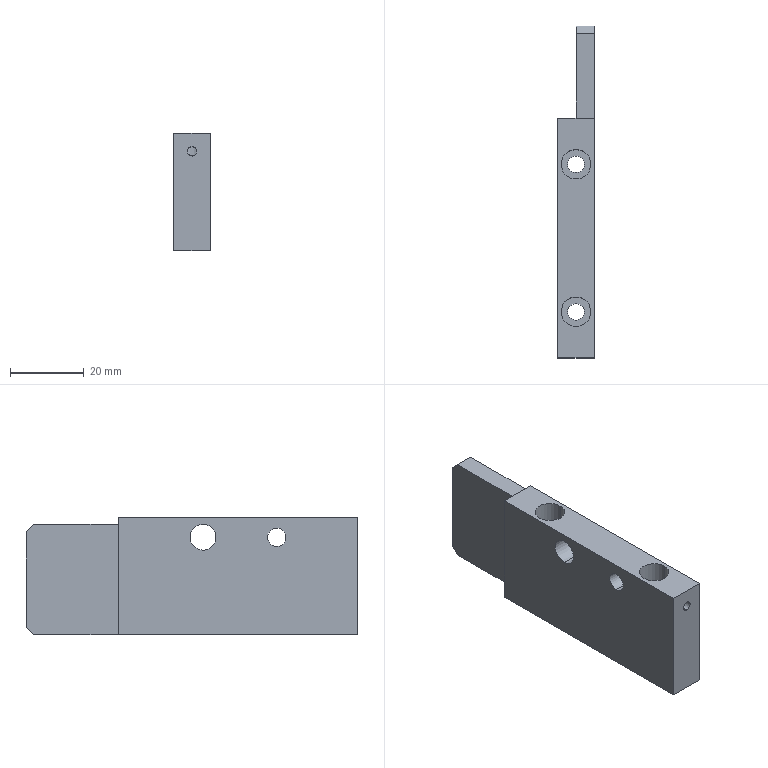Part | STEP file | PN_0064 Mount electronic clip s horizontal manipulator cylinder seat | 1 solid | 30 faces | box 10 x 90 x 32 mm | volume 21348 mm3 | cylinder 16 | plane 14 | commonest cylinder face diameters 2.5 x4 4.5 x4 8 x4 5 x2 7 x2